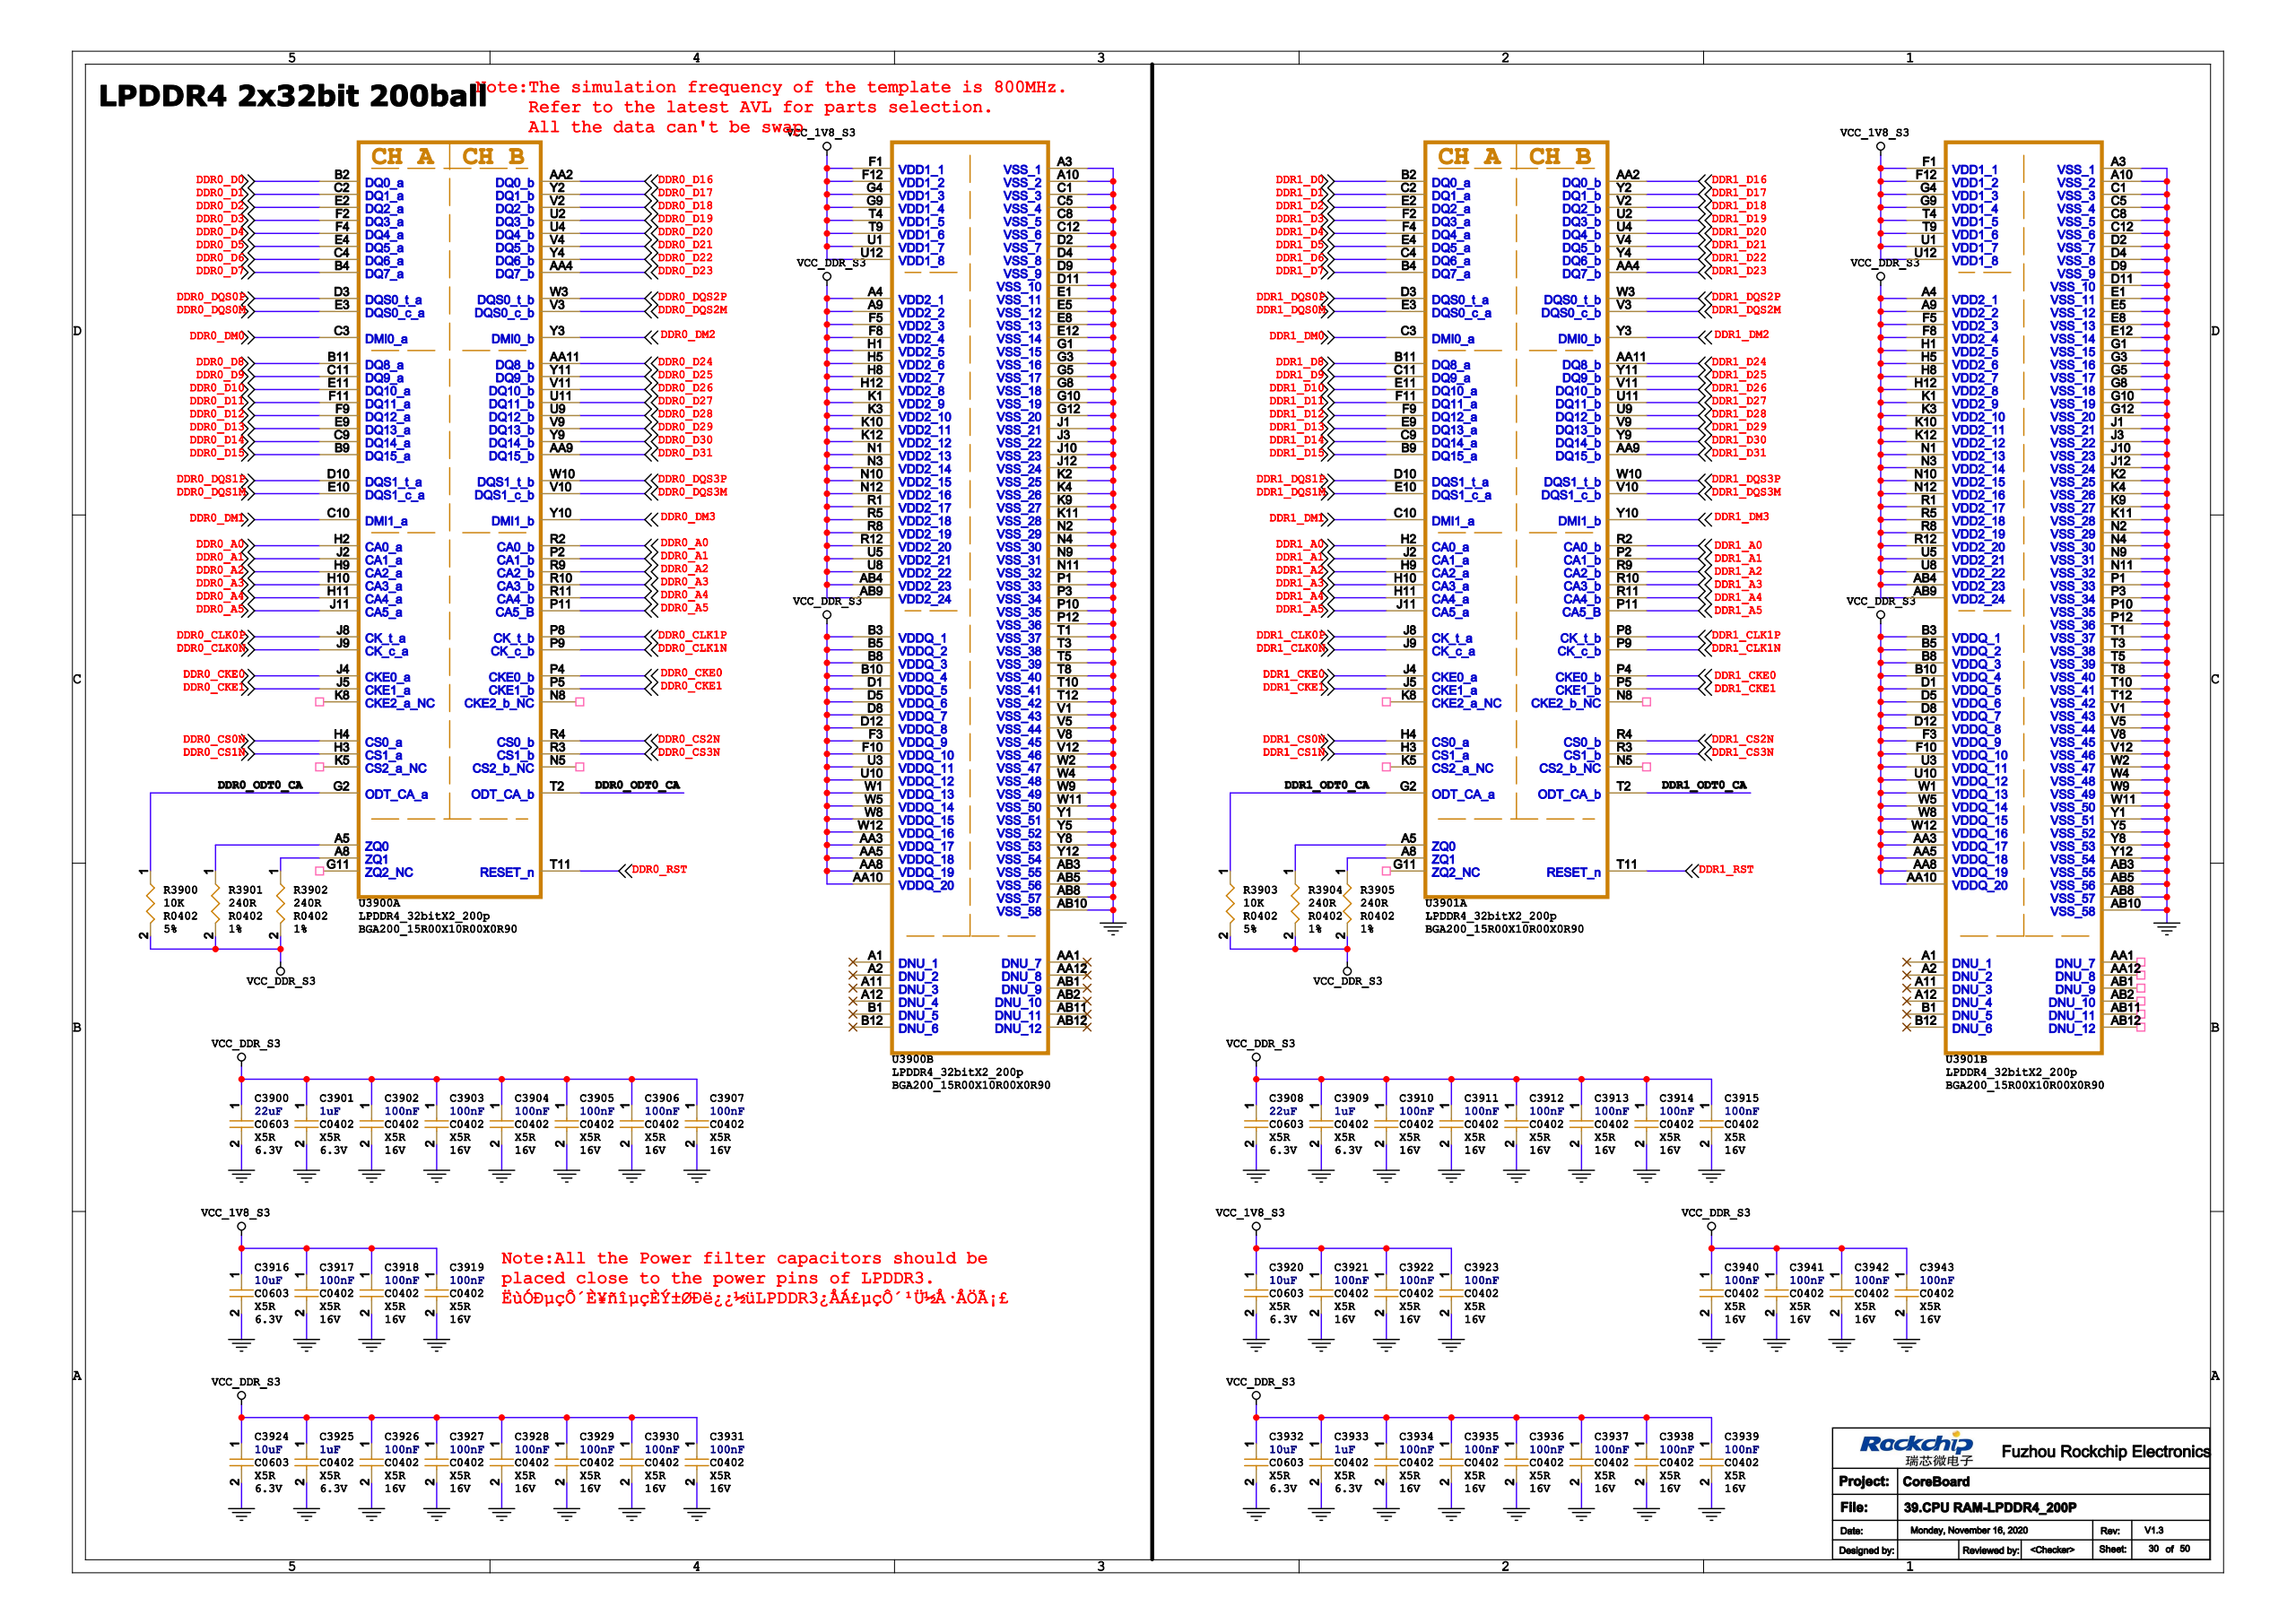Circuit board | Cadence Allegro | 749 parts | 717 nets | one sheet of the schematic
Parts on this sheet (reference | value | footprint):
C3900 | 22uF | C0603
C3901 | 1uF | C0402
C3902 | 100nF | C0402
C3903 | 100nF | C0402
C3904 | 100nF | C0402
C3905 | 100nF | C0402
C3906 | 100nF | C0402
C3907 | 100nF | C0402
C3908 | 22uF | C0603
C3909 | 1uF | C0402
C3910 | 100nF | C0402
C3911 | 100nF | C0402
C3912 | 100nF | C0402
C3913 | 100nF | C0402
C3914 | 100nF | C0402
C3915 | 100nF | C0402
C3916 | 10uF | C0603
C3917 | 100nF | C0402
C3918 | 100nF | C0402
C3919 | 100nF | C0402
C3920 | 10uF | C0603
C3921 | 100nF | C0402
C3922 | 100nF | C0402
C3923 | 100nF | C0402
C3924 | 10uF | C0603
C3925 | 1uF | C0402
C3926 | 100nF | C0402
C3927 | 100nF | C0402
C3928 | 100nF | C0402
C3929 | 100nF | C0402
C3930 | 100nF | C0402
C3931 | 100nF | C0402
C3932 | 10uF | C0603
C3933 | 1uF | C0402
C3934 | 100nF | C0402
C3935 | 100nF | C0402
C3936 | 100nF | C0402
C3937 | 100nF | C0402
C3938 | 100nF | C0402
C3939 | 100nF | C0402
C3940 | 100nF | C0402
C3941 | 100nF | C0402
C3942 | 100nF | C0402
C3943 | 100nF | C0402
R3900 | 10K | R0402
R3901 | 240R | R0402
R3902 | 240R | R0402
R3903 | 10K | R0402
R3904 | 240R | R0402
R3905 | 240R | R0402
U3900 | LPDDR4_32bitX2_200p | BGA200_15R00X10R00X0R90
U3901 | LPDDR4_32bitX2_200p | BGA200_15R00X10R00X0R90
Nets of these parts (net: part-pin ...):
GND: C3900-2 C3901-2 C3902-2 C3903-2 C3904-2 C3905-2 C3906-2 C3907-2 C3908-2 C3909-2 C3910-2 C3911-2 C3912-2 C3913-2 C3914-2 C3915-2 C3916-2 C3917-2 C3918-2 C3919-2 C3920-2 C3921-2 C3922-2 C3923-2 C3924-2 C3925-2 C3926-2 C3927-2 C3928-2 C3929-2 C3930-2 C3931-2 C3932-2 C3933-2 C3934-2 C3935-2 C3936-2 C3937-2 C3938-2 C3939-2 C3940-2 C3941-2 C3942-2 C3943-2 U3900-A3 U3900-A10 U3900-AB3 U3900-AB5 U3900-AB8 U3900-AB10 U3900-C1 U3900-C5 U3900-C8 U3900-C12 U3900-D2 U3900-D4 U3900-D9 U3900-D11 U3900-E1 U3900-E5 U3900-E8 U3900-E12 U3900-G1 U3900-G3 U3900-G5 U3900-G8 U3900-G10 U3900-G12 U3900-J1 U3900-J3 U3900-J10 U3900-J12 U3900-K2 U3900-K4 U3900-K9 U3900-K11 U3900-N2 U3900-N4 U3900-N9 U3900-N11 U3900-P1 U3900-P3 U3900-P10 U3900-P12 U3900-T1 U3900-T3 U3900-T5 U3900-T8 U3900-T10 U3900-T12 U3900-V1 U3900-V5 U3900-V8 U3900-V12 U3900-W2 U3900-W4 U3900-W9 U3900-W11 U3900-Y1 U3900-Y5 U3900-Y8 U3900-Y12 U3901-A3 U3901-A10 U3901-AB3 U3901-AB5 U3901-AB8 U3901-AB10 U3901-C1 U3901-C5 U3901-C8 U3901-C12 U3901-D2 U3901-D4 U3901-D9 U3901-D11 U3901-E1 U3901-E5 U3901-E8 U3901-E12 U3901-G1 U3901-G3 U3901-G5 U3901-G8 U3901-G10 U3901-G12 U3901-J1 U3901-J3 U3901-J10 U3901-J12 U3901-K2 U3901-K4 U3901-K9 U3901-K11 U3901-N2 U3901-N4 U3901-N9 U3901-N11 U3901-P1 U3901-P3 U3901-P10 U3901-P12 U3901-T1 U3901-T3 U3901-T5 U3901-T8 U3901-T10 U3901-T12 U3901-V1 U3901-V5 U3901-V8 U3901-V12 U3901-W2 U3901-W4 U3901-W9 U3901-W11 U3901-Y1 U3901-Y5 U3901-Y8 U3901-Y12
VCC_DDR_S3: C3900-1 C3901-1 C3902-1 C3903-1 C3904-1 C3905-1 C3906-1 C3907-1 C3908-1 C3909-1 C3910-1 C3911-1 C3912-1 C3913-1 C3914-1 C3915-1 C3924-1 C3925-1 C3926-1 C3927-1 C3928-1 C3929-1 C3930-1 C3931-1 C3932-1 C3933-1 C3934-1 C3935-1 C3936-1 C3937-1 C3938-1 C3939-1 C3940-1 C3941-1 C3942-1 C3943-1 R3900-2 R3901-2 R3902-2 R3903-2 R3904-2 R3905-2 U3900-A4 U3900-A9 U3900-AA3 U3900-AA5 U3900-AA8 U3900-AA10 U3900-AB4 U3900-AB9 U3900-B3 U3900-B5 U3900-B8 U3900-B10 U3900-D1 U3900-D5 U3900-D8 U3900-D12 U3900-F3 U3900-F5 U3900-F8 U3900-F10 U3900-H1 U3900-H5 U3900-H8 U3900-H12 U3900-K1 U3900-K3 U3900-K10 U3900-K12 U3900-N1 U3900-N3 U3900-N10 U3900-N12 U3900-R1 U3900-R5 U3900-R8 U3900-R12 U3900-U3 U3900-U5 U3900-U8 U3900-U10 U3900-W1 U3900-W5 U3900-W8 U3900-W12 U3901-A4 U3901-A9 U3901-AA3 U3901-AA5 U3901-AA8 U3901-AA10 U3901-AB4 U3901-AB9 U3901-B3 U3901-B5 U3901-B8 U3901-B10 U3901-D1 U3901-D5 U3901-D8 U3901-D12 U3901-F3 U3901-F5 U3901-F8 U3901-F10 U3901-H1 U3901-H5 U3901-H8 U3901-H12 U3901-K1 U3901-K3 U3901-K10 U3901-K12 U3901-N1 U3901-N3 U3901-N10 U3901-N12 U3901-R1 U3901-R5 U3901-R8 U3901-R12 U3901-U3 U3901-U5 U3901-U8 U3901-U10 U3901-W1 U3901-W5 U3901-W8 U3901-W12
VCC_1V8_S3: C3916-1 C3917-1 C3918-1 C3919-1 C3920-1 C3921-1 C3922-1 C3923-1 U3900-F1 U3900-F12 U3900-G4 U3900-G9 U3900-T4 U3900-T9 U3900-U1 U3900-U12 U3901-F1 U3901-F12 U3901-G4 U3901-G9 U3901-T4 U3901-T9 U3901-U1 U3901-U12
DDR0_A0: U3900-H2 U3900-R2
DDR0_A1: U3900-J2 U3900-P2
DDR0_A2: U3900-H9 U3900-R9
DDR0_A3: U3900-H10 U3900-R10
DDR0_A4: U3900-H11 U3900-R11
DDR0_A5: U3900-J11 U3900-P11
DDR0_CKE0: U3900-J4 U3900-P4
DDR0_CKE1: U3900-J5 U3900-P5
DDR0_CLK0N: U3900-J9
DDR0_CLK0P: U3900-J8
DDR0_CLK1N: U3900-P9
DDR0_CLK1P: U3900-P8
DDR0_CS0N: U3900-H4
DDR0_CS1N: U3900-H3
DDR0_CS2N: U3900-R4
DDR0_CS3N: U3900-R3
DDR0_DM0: U3900-C3
DDR0_DM1: U3900-C10
DDR0_DM2: U3900-Y3
DDR0_DM3: U3900-Y10
DDR0_D0: U3900-B2
DDR0_D1: U3900-C2
DDR0_D10: U3900-E11
DDR0_D11: U3900-F11
DDR0_D12: U3900-F9
DDR0_D13: U3900-E9
DDR0_D14: U3900-C9
DDR0_D15: U3900-B9
DDR0_D16: U3900-AA2
DDR0_D17: U3900-Y2
DDR0_D18: U3900-V2
DDR0_D19: U3900-U2
DDR0_D2: U3900-E2
DDR0_D20: U3900-U4
DDR0_D21: U3900-V4
DDR0_D22: U3900-Y4
DDR0_D23: U3900-AA4
DDR0_D24: U3900-AA11
DDR0_D25: U3900-Y11
DDR0_D26: U3900-V11
DDR0_D27: U3900-U11
DDR0_D28: U3900-U9
DDR0_D29: U3900-V9
DDR0_D3: U3900-F2
DDR0_D30: U3900-Y9
DDR0_D31: U3900-AA9
DDR0_D4: U3900-F4
DDR0_D5: U3900-E4
DDR0_D6: U3900-C4
DDR0_D7: U3900-B4
DDR0_D8: U3900-B11
DDR0_D9: U3900-C11
DDR0_DQS0M: U3900-E3
DDR0_DQS0P: U3900-D3
DDR0_DQS1M: U3900-E10
DDR0_DQS1P: U3900-D10
DDR0_DQS2M: U3900-V3
DDR0_DQS2P: U3900-W3
DDR0_DQS3M: U3900-V10
DDR0_DQS3P: U3900-W10
DDR0_RST: U3900-T11
DDR1_A0: U3901-H2 U3901-R2
DDR1_A1: U3901-J2 U3901-P2
DDR1_A2: U3901-H9 U3901-R9
DDR1_A3: U3901-H10 U3901-R10
DDR1_A4: U3901-H11 U3901-R11
DDR1_A5: U3901-J11 U3901-P11
DDR1_CKE0: U3901-J4 U3901-P4
DDR1_CKE1: U3901-J5 U3901-P5
DDR1_CLK0N: U3901-J9
DDR1_CLK0P: U3901-J8
DDR1_CLK1N: U3901-P9
DDR1_CLK1P: U3901-P8
DDR1_CS0N: U3901-H4
DDR1_CS1N: U3901-H3
DDR1_CS2N: U3901-R4
DDR1_CS3N: U3901-R3
DDR1_DM0: U3901-C3
DDR1_DM1: U3901-C10
DDR1_DM2: U3901-Y3
DDR1_DM3: U3901-Y10
DDR1_D0: U3901-B2
DDR1_D1: U3901-C2
DDR1_D10: U3901-E11
DDR1_D11: U3901-F11
DDR1_D12: U3901-F9
DDR1_D13: U3901-E9
DDR1_D14: U3901-C9
DDR1_D15: U3901-B9
DDR1_D16: U3901-AA2
DDR1_D17: U3901-Y2
DDR1_D18: U3901-V2
DDR1_D19: U3901-U2
DDR1_D2: U3901-E2
DDR1_D20: U3901-U4
DDR1_D21: U3901-V4
DDR1_D22: U3901-Y4
DDR1_D23: U3901-AA4
DDR1_D24: U3901-AA11
DDR1_D25: U3901-Y11
DDR1_D26: U3901-V11
DDR1_D27: U3901-U11
DDR1_D28: U3901-U9
DDR1_D29: U3901-V9
DDR1_D3: U3901-F2
DDR1_D30: U3901-Y9
DDR1_D31: U3901-AA9
DDR1_D4: U3901-F4
DDR1_D5: U3901-E4
DDR1_D6: U3901-C4
DDR1_D7: U3901-B4
DDR1_D8: U3901-B11
DDR1_D9: U3901-C11
DDR1_DQS0M: U3901-E3
DDR1_DQS0P: U3901-D3
DDR1_DQS1M: U3901-E10
DDR1_DQS1P: U3901-D10
DDR1_DQS2M: U3901-V3
DDR1_DQS2P: U3901-W3
DDR1_DQS3M: U3901-V10
DDR1_DQS3P: U3901-W10
DDR1_RST: U3901-T11
DDR0_ODT0_CA: R3900-1 U3900-G2 U3900-T2
N16865266: R3901-1 U3900-A5
N16870799: R3902-1 U3900-A8
DDR1_ODT0_CA: R3903-1 U3901-G2 U3901-T2
N16873503: R3904-1 U3901-A5
N16875336: R3905-1 U3901-A8